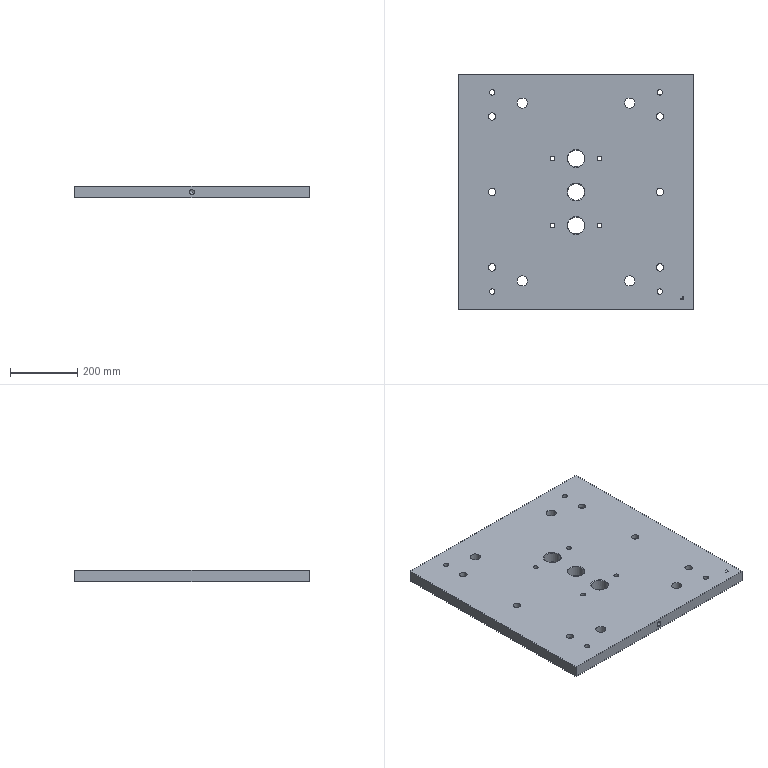Part | NX | features 模具.stp<1>[11] 2 | 1 solid | 92 faces | box 700 x 700 x 35 mm | volume 16617949 mm3 | cylinder 45 | plane 39 | cone 8 | commonest cylinder face diameters 16 x6 22 x6 32 x6 14 x4 20 x4 23 x4